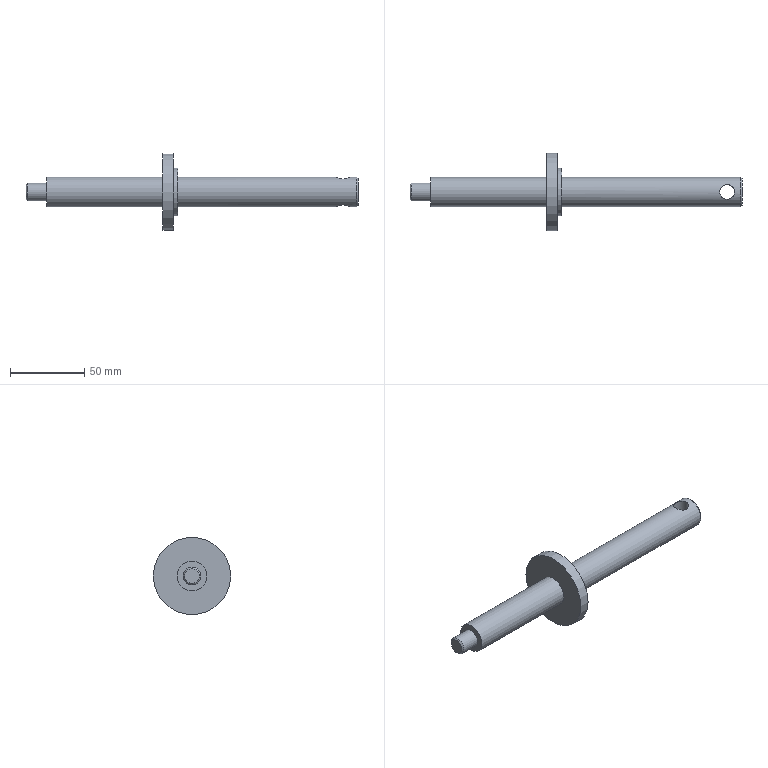Part | NX | features DATUM_CSYS 3, SKETCH 2, CHAMFER 1, EXTRUDE 1, HOLE PACKAGE 1, SIMPLE HOLE 1, SWP104 1, SYMBOLIC_THREAD 1 | 1 solid | 17 faces | box 223 x 52 x 52 mm | volume 79707 mm3 | cylinder 7 | plane 6 | cone 3 | spline 1 | commonest cylinder face diameters 20 x2 5 x1 10 x1 12 x1 32 x1 52 x1
STEP:
#1=CARTESIAN_POINT('',(222.,-10.,0.));
#2=VERTEX_POINT('',#1);
#3=CARTESIAN_POINT('',(222.,0.,0.));
#4=DIRECTION('',(-1.,0.,0.));
#5=DIRECTION('',(0.,-1.,0.));
#6=AXIS2_PLACEMENT_3D('',#3,#4,#5);
#7=CIRCLE('',#6,10.);
#8=EDGE_CURVE('',#2,#2,#7,.T.);
#9=ORIENTED_EDGE('',*,*,#8,.T.);
#10=EDGE_LOOP('',(#9));
#11=FACE_BOUND('',#10,.T.);
#12=CARTESIAN_POINT('',(102.,10.,0.));
#13=VERTEX_POINT('',#12);
#14=CARTESIAN_POINT('',(102.,0.,0.));
#15=DIRECTION('',(1.,0.,0.));
#16=DIRECTION('',(0.,1.,0.));
#17=AXIS2_PLACEMENT_3D('',#14,#15,#16);
#18=CIRCLE('',#17,10.);
#19=EDGE_CURVE('',#13,#13,#18,.T.);
#20=ORIENTED_EDGE('',*,*,#19,.T.);
#21=EDGE_LOOP('',(#20));
#22=FACE_BOUND('',#21,.T.);
#23=CARTESIAN_POINT('',(208.,0.,-10.));
#24=VERTEX_POINT('',#23);
#25=CARTESIAN_POINT('',(208.277,-2.001,-9.858));
#26=CARTESIAN_POINT('',(207.724,0.6768,-10.148));
#27=CARTESIAN_POINT('',(209.099,3.912,-9.377));
#28=CARTESIAN_POINT('',(212.31,5.272,-8.49));
#29=CARTESIAN_POINT('',(214.988,4.729,-8.824));
#30=CARTESIAN_POINT('',(217.159,3.276,-9.538));
#31=CARTESIAN_POINT('',(218.551,0.01854,-10.309));
#32=CARTESIAN_POINT('',(216.914,-3.918,-9.379));
#33=CARTESIAN_POINT('',(213.019,-5.545,-8.305));
#34=CARTESIAN_POINT('',(209.738,-4.174,-9.187));
#35=CARTESIAN_POINT('',(208.277,-2.001,-9.858));
#36=CARTESIAN_POINT('',(207.724,0.6768,-10.148));
#37=CARTESIAN_POINT('',(209.099,3.912,-9.377));
#38=B_SPLINE_CURVE_WITH_KNOTS('',3,(#25,#26,#27,#28,#29,#30,#31,#32,#33,#34,#35,#36,#37),.UNSPECIFIED.,.T.,.F.,(1,1,1,1,1,1,1,1,1,1,1,1,1,1,1,1,1),(-0.007946,-0.003973,-0.001986,0.,0.003973,0.007946,0.009932,0.01192,0.01589,0.01986,0.02384,0.02781,0.0298,0.03178,0.03575,0.03973,0.04171),.UNSPECIFIED.);
#39=EDGE_CURVE('',#24,#24,#38,.T.);
#40=ORIENTED_EDGE('',*,*,#39,.F.);
#41=EDGE_LOOP('',(#40));
#42=FACE_BOUND('',#41,.T.);
#43=CARTESIAN_POINT('',(208.,0.,10.));
#44=VERTEX_POINT('',#43);
#45=CARTESIAN_POINT('',(208.277,2.001,9.858));
#46=CARTESIAN_POINT('',(207.724,-0.6768,10.148));
#47=CARTESIAN_POINT('',(209.099,-3.912,9.377));
#48=CARTESIAN_POINT('',(212.31,-5.272,8.49));
#49=CARTESIAN_POINT('',(214.988,-4.729,8.824));
#50=CARTESIAN_POINT('',(217.159,-3.276,9.538));
#51=CARTESIAN_POINT('',(218.551,-0.01854,10.309));
#52=CARTESIAN_POINT('',(216.914,3.918,9.379));
#53=CARTESIAN_POINT('',(213.019,5.545,8.305));
#54=CARTESIAN_POINT('',(209.738,4.174,9.187));
#55=CARTESIAN_POINT('',(208.277,2.001,9.858));
#56=CARTESIAN_POINT('',(207.724,-0.6768,10.148));
#57=CARTESIAN_POINT('',(209.099,-3.912,9.377));
#58=B_SPLINE_CURVE_WITH_KNOTS('',3,(#45,#46,#47,#48,#49,#50,#51,#52,#53,#54,#55,#56,#57),.UNSPECIFIED.,.T.,.F.,(1,1,1,1,1,1,1,1,1,1,1,1,1,1,1,1,1),(-0.007946,-0.003973,-0.001986,0.,0.003973,0.007946,0.009932,0.01192,0.01589,0.01986,0.02384,0.02781,0.0298,0.03178,0.03575,0.03973,0.04171),.UNSPECIFIED.);
#59=EDGE_CURVE('',#44,#44,#58,.T.);
#60=ORIENTED_EDGE('',*,*,#59,.F.);
#61=EDGE_LOOP('',(#60));
#62=FACE_BOUND('',#61,.T.);
#63=CARTESIAN_POINT('',(0.,0.,0.));
#64=DIRECTION('',(1.,0.,0.));
#65=DIRECTION('',(0.,1.,0.));
#66=AXIS2_PLACEMENT_3D('',#63,#64,#65);
#67=CYLINDRICAL_SURFACE('',#66,10.);
#68=ADVANCED_FACE('',(#11,#22,#42,#62),#67,.T.);
#69=CARTESIAN_POINT('',(0.,5.,0.));
#70=VERTEX_POINT('',#69);
#71=CARTESIAN_POINT('',(0.,0.,0.));
#72=DIRECTION('',(1.,0.,0.));
#73=DIRECTION('',(0.,1.,0.));
#74=AXIS2_PLACEMENT_3D('',#71,#72,#73);
#75=CIRCLE('',#74,5.);
#76=EDGE_CURVE('',#70,#70,#75,.F.);
#77=ORIENTED_EDGE('',*,*,#76,.T.);
#78=EDGE_LOOP('',(#77));
#79=FACE_BOUND('',#78,.T.);
#80=CARTESIAN_POINT('',(0.,0.,0.));
#81=DIRECTION('',(1.,0.,0.));
#82=DIRECTION('',(0.,1.,0.));
#83=AXIS2_PLACEMENT_3D('',#80,#81,#82);
#84=PLANE('',#83);
#85=ADVANCED_FACE('',(#79),#84,.F.);
#86=CARTESIAN_POINT('',(1.,6.,0.));
#87=VERTEX_POINT('',#86);
#88=CARTESIAN_POINT('',(1.,0.,0.));
#89=DIRECTION('',(1.,0.,0.));
#90=DIRECTION('',(0.,1.,0.));
#91=AXIS2_PLACEMENT_3D('',#88,#89,#90);
#92=CIRCLE('',#91,6.);
#93=EDGE_CURVE('',#87,#87,#92,.T.);
#94=ORIENTED_EDGE('',*,*,#93,.T.);
#95=EDGE_LOOP('',(#94));
#96=FACE_BOUND('',#95,.T.);
#97=CARTESIAN_POINT('',(14.,6.,0.));
#98=VERTEX_POINT('',#97);
#99=CARTESIAN_POINT('',(14.,0.,0.));
#100=DIRECTION('',(1.,0.,0.));
#101=DIRECTION('',(0.,1.,0.));
#102=AXIS2_PLACEMENT_3D('',#99,#100,#101);
#103=CIRCLE('',#102,6.);
#104=EDGE_CURVE('',#98,#98,#103,.T.);
#105=ORIENTED_EDGE('',*,*,#104,.F.);
#106=EDGE_LOOP('',(#105));
#107=FACE_BOUND('',#106,.T.);
#108=CARTESIAN_POINT('',(0.,0.,0.));
#109=DIRECTION('',(1.,0.,0.));
#110=DIRECTION('',(0.,1.,0.));
#111=AXIS2_PLACEMENT_3D('',#108,#109,#110);
#112=CYLINDRICAL_SURFACE('',#111,6.);
#113=ADVANCED_FACE('',(#96,#107),#112,.T.);
#114=CARTESIAN_POINT('',(14.,10.,0.));
#115=VERTEX_POINT('',#114);
#116=CARTESIAN_POINT('',(14.,0.,0.));
#117=DIRECTION('',(1.,0.,0.));
#118=DIRECTION('',(0.,1.,0.));
#119=AXIS2_PLACEMENT_3D('',#116,#117,#118);
#120=CIRCLE('',#119,10.);
#121=EDGE_CURVE('',#115,#115,#120,.T.);
#122=ORIENTED_EDGE('',*,*,#121,.F.);
#123=EDGE_LOOP('',(#122));
#124=FACE_BOUND('',#123,.T.);
#125=ORIENTED_EDGE('',*,*,#104,.T.);
#126=EDGE_LOOP('',(#125));
#127=FACE_BOUND('',#126,.T.);
#128=CARTESIAN_POINT('',(14.,6.,0.));
#129=DIRECTION('',(1.,0.,0.));
#130=DIRECTION('',(0.,1.,0.));
#131=AXIS2_PLACEMENT_3D('',#128,#129,#130);
#132=PLANE('',#131);
#133=ADVANCED_FACE('',(#124,#127),#132,.F.);
#134=CARTESIAN_POINT('',(92.,10.,0.));
#135=VERTEX_POINT('',#134);
#136=CARTESIAN_POINT('',(92.,0.,0.));
#137=DIRECTION('',(1.,0.,0.));
#138=DIRECTION('',(0.,1.,0.));
#139=AXIS2_PLACEMENT_3D('',#136,#137,#138);
#140=CIRCLE('',#139,10.);
#141=EDGE_CURVE('',#135,#135,#140,.T.);
#142=ORIENTED_EDGE('',*,*,#141,.F.);
#143=EDGE_LOOP('',(#142));
#144=FACE_BOUND('',#143,.T.);
#145=ORIENTED_EDGE('',*,*,#121,.T.);
#146=EDGE_LOOP('',(#145));
#147=FACE_BOUND('',#146,.T.);
#148=CARTESIAN_POINT('',(0.,0.,0.));
#149=DIRECTION('',(1.,0.,0.));
#150=DIRECTION('',(0.,1.,0.));
#151=AXIS2_PLACEMENT_3D('',#148,#149,#150);
#152=CYLINDRICAL_SURFACE('',#151,10.);
#153=ADVANCED_FACE('',(#144,#147),#152,.T.);
#154=CARTESIAN_POINT('',(92.,26.,0.));
#155=VERTEX_POINT('',#154);
#156=CARTESIAN_POINT('',(92.,0.,0.));
#157=DIRECTION('',(1.,0.,0.));
#158=DIRECTION('',(0.,1.,0.));
#159=AXIS2_PLACEMENT_3D('',#156,#157,#158);
#160=CIRCLE('',#159,26.);
#161=EDGE_CURVE('',#155,#155,#160,.T.);
#162=ORIENTED_EDGE('',*,*,#161,.F.);
#163=EDGE_LOOP('',(#162));
#164=FACE_BOUND('',#163,.T.);
#165=ORIENTED_EDGE('',*,*,#141,.T.);
#166=EDGE_LOOP('',(#165));
#167=FACE_BOUND('',#166,.T.);
#168=CARTESIAN_POINT('',(92.,10.,0.));
#169=DIRECTION('',(1.,0.,0.));
#170=DIRECTION('',(0.,1.,0.));
#171=AXIS2_PLACEMENT_3D('',#168,#169,#170);
#172=PLANE('',#171);
#173=ADVANCED_FACE('',(#164,#167),#172,.F.);
#174=CARTESIAN_POINT('',(99.,26.,0.));
#175=VERTEX_POINT('',#174);
#176=CARTESIAN_POINT('',(99.,0.,0.));
#177=DIRECTION('',(1.,0.,0.));
#178=DIRECTION('',(0.,1.,0.));
#179=AXIS2_PLACEMENT_3D('',#176,#177,#178);
#180=CIRCLE('',#179,26.);
#181=EDGE_CURVE('',#175,#175,#180,.T.);
#182=ORIENTED_EDGE('',*,*,#181,.F.);
#183=EDGE_LOOP('',(#182));
#184=FACE_BOUND('',#183,.T.);
#185=ORIENTED_EDGE('',*,*,#161,.T.);
#186=EDGE_LOOP('',(#185));
#187=FACE_BOUND('',#186,.T.);
#188=CARTESIAN_POINT('',(0.,0.,0.));
#189=DIRECTION('',(1.,0.,0.));
#190=DIRECTION('',(0.,1.,0.));
#191=AXIS2_PLACEMENT_3D('',#188,#189,#190);
#192=CYLINDRICAL_SURFACE('',#191,26.);
#193=ADVANCED_FACE('',(#184,#187),#192,.T.);
#194=CARTESIAN_POINT('',(99.,16.,0.));
#195=VERTEX_POINT('',#194);
#196=CARTESIAN_POINT('',(99.,0.,0.));
#197=DIRECTION('',(1.,0.,0.));
#198=DIRECTION('',(0.,1.,0.));
#199=AXIS2_PLACEMENT_3D('',#196,#197,#198);
#200=CIRCLE('',#199,16.);
#201=EDGE_CURVE('',#195,#195,#200,.T.);
#202=ORIENTED_EDGE('',*,*,#201,.F.);
#203=EDGE_LOOP('',(#202));
#204=FACE_BOUND('',#203,.T.);
#205=ORIENTED_EDGE('',*,*,#181,.T.);
#206=EDGE_LOOP('',(#205));
#207=FACE_BOUND('',#206,.T.);
#208=CARTESIAN_POINT('',(99.,26.,0.));
#209=DIRECTION('',(-1.,0.,0.));
#210=DIRECTION('',(0.,-1.,0.));
#211=AXIS2_PLACEMENT_3D('',#208,#209,#210);
#212=PLANE('',#211);
#213=ADVANCED_FACE('',(#204,#207),#212,.F.);
#214=CARTESIAN_POINT('',(102.,16.,0.));
#215=VERTEX_POINT('',#214);
#216=CARTESIAN_POINT('',(102.,0.,0.));
#217=DIRECTION('',(1.,0.,0.));
#218=DIRECTION('',(0.,1.,0.));
#219=AXIS2_PLACEMENT_3D('',#216,#217,#218);
#220=CIRCLE('',#219,16.);
#221=EDGE_CURVE('',#215,#215,#220,.T.);
#222=ORIENTED_EDGE('',*,*,#221,.F.);
#223=EDGE_LOOP('',(#222));
#224=FACE_BOUND('',#223,.T.);
#225=ORIENTED_EDGE('',*,*,#201,.T.);
#226=EDGE_LOOP('',(#225));
#227=FACE_BOUND('',#226,.T.);
#228=CARTESIAN_POINT('',(0.,0.,0.));
#229=DIRECTION('',(1.,0.,0.));
#230=DIRECTION('',(0.,1.,0.));
#231=AXIS2_PLACEMENT_3D('',#228,#229,#230);
#232=CYLINDRICAL_SURFACE('',#231,16.);
#233=ADVANCED_FACE('',(#224,#227),#232,.T.);
#234=ORIENTED_EDGE('',*,*,#19,.F.);
#235=EDGE_LOOP('',(#234));
#236=FACE_BOUND('',#235,.T.);
#237=ORIENTED_EDGE('',*,*,#221,.T.);
#238=EDGE_LOOP('',(#237));
#239=FACE_BOUND('',#238,.T.);
#240=CARTESIAN_POINT('',(102.,16.,0.));
#241=DIRECTION('',(-1.,0.,0.));
#242=DIRECTION('',(0.,-1.,0.));
#243=AXIS2_PLACEMENT_3D('',#240,#241,#242);
#244=PLANE('',#243);
#245=ADVANCED_FACE('',(#236,#239),#244,.F.);
#246=CARTESIAN_POINT('',(223.,-3.,0.));
#247=VERTEX_POINT('',#246);
#248=CARTESIAN_POINT('',(223.,0.,0.));
#249=DIRECTION('',(-1.,0.,0.));
#250=DIRECTION('',(0.,-1.,0.));
#251=AXIS2_PLACEMENT_3D('',#248,#249,#250);
#252=CIRCLE('',#251,3.);
#253=EDGE_CURVE('',#247,#247,#252,.T.);
#254=ORIENTED_EDGE('',*,*,#253,.T.);
#255=EDGE_LOOP('',(#254));
#256=FACE_BOUND('',#255,.T.);
#257=CARTESIAN_POINT('',(223.,-9.,0.));
#258=VERTEX_POINT('',#257);
#259=CARTESIAN_POINT('',(223.,0.,0.));
#260=DIRECTION('',(-1.,0.,0.));
#261=DIRECTION('',(0.,-1.,0.));
#262=AXIS2_PLACEMENT_3D('',#259,#260,#261);
#263=CIRCLE('',#262,9.);
#264=EDGE_CURVE('',#258,#258,#263,.F.);
#265=ORIENTED_EDGE('',*,*,#264,.T.);
#266=EDGE_LOOP('',(#265));
#267=FACE_BOUND('',#266,.T.);
#268=CARTESIAN_POINT('',(223.,10.,0.));
#269=DIRECTION('',(-1.,0.,0.));
#270=DIRECTION('',(0.,-1.,0.));
#271=AXIS2_PLACEMENT_3D('',#268,#269,#270);
#272=PLANE('',#271);
#273=ADVANCED_FACE('',(#256,#267),#272,.F.);
#274=ORIENTED_EDGE('',*,*,#8,.F.);
#275=EDGE_LOOP('',(#274));
#276=FACE_BOUND('',#275,.T.);
#277=ORIENTED_EDGE('',*,*,#264,.F.);
#278=EDGE_LOOP('',(#277));
#279=FACE_BOUND('',#278,.T.);
#280=CARTESIAN_POINT('',(223.,0.,0.));
#281=DIRECTION('',(-1.,0.,0.));
#282=DIRECTION('',(0.,-1.,0.));
#283=AXIS2_PLACEMENT_3D('',#280,#281,#282);
#284=CONICAL_SURFACE('',#283,9.,0.7854);
#285=ADVANCED_FACE('',(#276,#279),#284,.T.);
#286=ORIENTED_EDGE('',*,*,#76,.F.);
#287=EDGE_LOOP('',(#286));
#288=FACE_BOUND('',#287,.T.);
#289=ORIENTED_EDGE('',*,*,#93,.F.);
#290=EDGE_LOOP('',(#289));
#291=FACE_BOUND('',#290,.T.);
#292=CARTESIAN_POINT('',(1.,0.,0.));
#293=DIRECTION('',(1.,0.,0.));
#294=DIRECTION('',(0.,1.,0.));
#295=AXIS2_PLACEMENT_3D('',#292,#293,#294);
#296=CONICAL_SURFACE('',#295,6.,0.7854);
#297=ADVANCED_FACE('',(#288,#291),#296,.T.);
#298=CARTESIAN_POINT('',(217.187,-2.733,0.));
#299=VERTEX_POINT('',#298);
#300=CARTESIAN_POINT('',(217.301,-2.566,1.32));
#301=CARTESIAN_POINT('',(217.134,-2.81,0.043));
#302=CARTESIAN_POINT('',(217.283,-2.593,-1.23));
#303=CARTESIAN_POINT('',(217.596,-2.024,-2.271));
#304=CARTESIAN_POINT('',(217.903,-1.148,-2.992));
#305=CARTESIAN_POINT('',(218.041,-0.06264,-3.292));
#306=CARTESIAN_POINT('',(217.93,1.032,-3.052));
#307=CARTESIAN_POINT('',(217.633,1.942,-2.368));
#308=CARTESIAN_POINT('',(217.308,2.554,-1.343));
#309=CARTESIAN_POINT('',(217.135,2.809,-0.07027));
#310=CARTESIAN_POINT('',(217.276,2.604,1.207));
#311=CARTESIAN_POINT('',(217.595,2.025,2.27));
#312=CARTESIAN_POINT('',(217.903,1.148,2.992));
#313=CARTESIAN_POINT('',(218.042,0.06158,3.292));
#314=CARTESIAN_POINT('',(217.929,-1.034,3.051));
#315=CARTESIAN_POINT('',(217.632,-1.944,2.366));
#316=CARTESIAN_POINT('',(217.301,-2.566,1.32));
#317=CARTESIAN_POINT('',(217.134,-2.81,0.043));
#318=CARTESIAN_POINT('',(217.283,-2.593,-1.23));
#319=B_SPLINE_CURVE_WITH_KNOTS('',3,(#300,#301,#302,#303,#304,#305,#306,#307,#308,#309,#310,#311,#312,#313,#314,#315,#316,#317,#318),.UNSPECIFIED.,.T.,.F.,(1,1,1,1,1,1,1,1,1,1,1,1,1,1,1,1,1,1,1,1,1,1,1),(-0.1908,-0.1283,-0.06579,0.,0.05937,0.1217,0.1842,0.2467,0.3092,0.3717,0.4342,0.4967,0.5592,0.6217,0.6842,0.7467,0.8092,0.8717,0.9342,1.,1.059,1.122,1.184),.UNSPECIFIED.);
#320=EDGE_CURVE('',#299,#299,#319,.T.);
#321=ORIENTED_EDGE('',*,*,#320,.T.);
#322=EDGE_LOOP('',(#321));
#323=FACE_BOUND('',#322,.T.);
#324=ORIENTED_EDGE('',*,*,#39,.T.);
#325=EDGE_LOOP('',(#324));
#326=FACE_BOUND('',#325,.T.);
#327=ORIENTED_EDGE('',*,*,#59,.T.);
#328=EDGE_LOOP('',(#327));
#329=FACE_BOUND('',#328,.T.);
#330=CARTESIAN_POINT('',(213.,0.,64.));
#331=DIRECTION('',(0.,0.,-1.));
#332=DIRECTION('',(-1.,0.,0.));
#333=AXIS2_PLACEMENT_3D('',#330,#331,#332);
#334=CYLINDRICAL_SURFACE('',#333,5.);
#335=ADVANCED_FACE('',(#323,#326,#329),#334,.F.);
#336=CARTESIAN_POINT('',(217.906,-2.5,0.));
#337=VERTEX_POINT('',#336);
#338=CARTESIAN_POINT('',(217.931,-2.476,-0.4847));
#339=CARTESIAN_POINT('',(217.895,-2.51,-0.01351));
#340=CARTESIAN_POINT('',(217.925,-2.482,0.4271));
#341=CARTESIAN_POINT('',(218.053,-2.32,0.9666));
#342=CARTESIAN_POINT('',(218.158,-2.177,1.253));
#343=CARTESIAN_POINT('',(218.451,-1.723,1.893));
#344=CARTESIAN_POINT('',(218.77,-0.9129,2.395));
#345=CARTESIAN_POINT('',(218.893,-0.06401,2.539));
#346=CARTESIAN_POINT('',(218.804,0.7449,2.442));
#347=CARTESIAN_POINT('',(218.538,1.561,2.039));
#348=CARTESIAN_POINT('',(218.198,2.121,1.357));
#349=CARTESIAN_POINT('',(218.078,2.286,1.043));
#350=CARTESIAN_POINT('',(217.937,2.468,0.5114));
#351=CARTESIAN_POINT('',(217.895,2.51,0.04032));
#352=CARTESIAN_POINT('',(217.92,2.488,-0.4006));
#353=CARTESIAN_POINT('',(218.051,2.322,-0.962));
#354=CARTESIAN_POINT('',(218.158,2.177,-1.254));
#355=CARTESIAN_POINT('',(218.452,1.721,-1.895));
#356=CARTESIAN_POINT('',(218.77,0.9117,-2.395));
#357=CARTESIAN_POINT('',(218.893,0.06296,-2.539));
#358=CARTESIAN_POINT('',(218.804,-0.7453,-2.441));
#359=CARTESIAN_POINT('',(218.538,-1.561,-2.039));
#360=CARTESIAN_POINT('',(218.199,-2.12,-1.358));
#361=CARTESIAN_POINT('',(218.076,-2.288,-1.039));
#362=CARTESIAN_POINT('',(217.931,-2.476,-0.4847));
#363=CARTESIAN_POINT('',(217.895,-2.51,-0.01351));
#364=CARTESIAN_POINT('',(217.925,-2.482,0.4271));
#365=B_SPLINE_CURVE_WITH_KNOTS('',3,(#338,#339,#340,#341,#342,#343,#344,#345,#346,#347,#348,#349,#350,#351,#352,#353,#354,#355,#356,#357,#358,#359,#360,#361,#362,#363,#364),.UNSPECIFIED.,.T.,.F.,(1,1,1,1,1,1,1,1,1,1,1,1,1,1,1,1,1,1,1,1,1,1,1,1,1,1,1,1,1,1,1),(-0.09876,-0.06595,-0.03298,0.,0.02969,0.05937,0.09055,0.1217,0.1827,0.2436,0.306,0.3684,0.4012,0.434,0.4654,0.4967,0.528,0.5592,0.5905,0.6217,0.6826,0.7436,0.806,0.8684,0.9012,0.934,0.967,1.,1.03,1.059,1.091),.UNSPECIFIED.);
#366=EDGE_CURVE('',#337,#337,#365,.T.);
#367=ORIENTED_EDGE('',*,*,#366,.T.);
#368=EDGE_LOOP('',(#367));
#369=FACE_BOUND('',#368,.T.);
#370=CARTESIAN_POINT('',(222.5,-2.5,0.));
#371=VERTEX_POINT('',#370);
#372=CARTESIAN_POINT('',(222.5,0.,0.));
#373=DIRECTION('',(-1.,0.,0.));
#374=DIRECTION('',(0.,-1.,0.));
#375=AXIS2_PLACEMENT_3D('',#372,#373,#374);
#376=CIRCLE('',#375,2.5);
#377=EDGE_CURVE('',#371,#371,#376,.F.);
#378=ORIENTED_EDGE('',*,*,#377,.T.);
#379=EDGE_LOOP('',(#378));
#380=FACE_BOUND('',#379,.T.);
#381=CARTESIAN_POINT('',(223.,0.,0.));
#382=DIRECTION('',(-1.,0.,0.));
#383=DIRECTION('',(0.,-1.,0.));
#384=AXIS2_PLACEMENT_3D('',#381,#382,#383);
#385=CYLINDRICAL_SURFACE('',#384,2.5);
#386=ADVANCED_FACE('',(#369,#380),#385,.F.);
#387=ORIENTED_EDGE('',*,*,#377,.F.);
#388=EDGE_LOOP('',(#387));
#389=FACE_BOUND('',#388,.T.);
#390=ORIENTED_EDGE('',*,*,#253,.F.);
#391=EDGE_LOOP('',(#390));
#392=FACE_BOUND('',#391,.T.);
#393=CARTESIAN_POINT('',(223.,0.,0.));
#394=DIRECTION('',(1.,0.,0.));
#395=DIRECTION('',(0.,1.,0.));
#396=AXIS2_PLACEMENT_3D('',#393,#394,#395);
#397=CONICAL_SURFACE('',#396,3.,0.7854);
#398=ADVANCED_FACE('',(#389,#392),#397,.F.);
#399=ORIENTED_EDGE('',*,*,#320,.F.);
#400=EDGE_LOOP('',(#399));
#401=FACE_BOUND('',#400,.T.);
#402=ORIENTED_EDGE('',*,*,#366,.F.);
#403=EDGE_LOOP('',(#402));
#404=FACE_BOUND('',#403,.T.);
#405=CARTESIAN_POINT('',(217.905,-2.501,-0.674));
#406=CARTESIAN_POINT('',(217.906,-2.499,0.674));
#407=CARTESIAN_POINT('',(218.156,-2.22,1.313));
#408=CARTESIAN_POINT('',(218.649,-1.319,2.219));
#409=CARTESIAN_POINT('',(218.86,-0.6705,2.501));
#410=CARTESIAN_POINT('',(218.858,0.6761,2.499));
#411=CARTESIAN_POINT('',(218.648,1.32,2.217));
#412=CARTESIAN_POINT('',(218.156,2.222,1.313));
#413=CARTESIAN_POINT('',(217.905,2.501,0.6725));
#414=CARTESIAN_POINT('',(217.907,2.499,-0.6778));
#415=CARTESIAN_POINT('',(218.158,2.218,-1.316));
#416=CARTESIAN_POINT('',(218.649,1.317,-2.22));
#417=CARTESIAN_POINT('',(218.86,0.6689,-2.502));
#418=CARTESIAN_POINT('',(218.857,-0.6764,-2.498));
#419=CARTESIAN_POINT('',(218.648,-1.319,-2.217));
#420=CARTESIAN_POINT('',(218.156,-2.221,-1.314));
#421=CARTESIAN_POINT('',(217.905,-2.501,-0.674));
#422=CARTESIAN_POINT('',(217.906,-2.499,0.674));
#423=CARTESIAN_POINT('',(217.186,-2.734,-0.8633));
#424=CARTESIAN_POINT('',(217.187,-2.732,0.8633));
#425=CARTESIAN_POINT('',(217.401,-2.427,1.682));
#426=CARTESIAN_POINT('',(217.821,-1.442,2.843));
#427=CARTESIAN_POINT('',(218.001,-0.7331,3.204));
#428=CARTESIAN_POINT('',(217.999,0.7392,3.201));
#429=CARTESIAN_POINT('',(217.82,1.443,2.84));
#430=CARTESIAN_POINT('',(217.4,2.429,1.682));
#431=CARTESIAN_POINT('',(217.186,2.735,0.8615));
#432=CARTESIAN_POINT('',(217.188,2.732,-0.8683));
#433=CARTESIAN_POINT('',(217.402,2.425,-1.686));
#434=CARTESIAN_POINT('',(217.821,1.44,-2.844));
#435=CARTESIAN_POINT('',(218.001,0.7313,-3.205));
#436=CARTESIAN_POINT('',(217.999,-0.7395,-3.2));
#437=CARTESIAN_POINT('',(217.82,-1.442,-2.84));
#438=CARTESIAN_POINT('',(217.401,-2.428,-1.683));
#439=CARTESIAN_POINT('',(217.186,-2.734,-0.8633));
#440=CARTESIAN_POINT('',(217.187,-2.732,0.8633));
#441=B_SPLINE_SURFACE_WITH_KNOTS('',1,3,((#405,#406,#407,#408,#409,#410,#411,#412,#413,#414,#415,#416,#417,#418,#419,#420,#421,#422),(#423,#424,#425,#426,#427,#428,#429,#430,#431,#432,#433,#434,#435,#436,#437,#438,#439,#440)),.RULED_SURF.,.F.,.T.,.F.,(2,2),(2,2,2,2,2,2,2,2,2,2,2),(0.,1.),(-0.02178,-0.01922,-0.01666,-0.01411,-0.01155,-0.008991,-0.006434,-0.003876,-0.001319,0.001238,0.003796),.UNSPECIFIED.);
#442=ADVANCED_FACE('',(#401,#404),#441,.T.);
#443=CLOSED_SHELL('',(#68,#85,#113,#133,#153,#173,#193,#213,#233,#245,#273,#285,#297,#335,#386,#398,#442));
#444=MANIFOLD_SOLID_BREP('',#443);
#445=(LENGTH_UNIT()NAMED_UNIT(*)SI_UNIT(.MILLI.,.METRE.));
#446=UNCERTAINTY_MEASURE_WITH_UNIT(LENGTH_MEASURE(0.0508),#445,'','');
#447=(NAMED_UNIT(*)PLANE_ANGLE_UNIT()SI_UNIT($,.RADIAN.));
#448=(NAMED_UNIT(*)SI_UNIT($,.STERADIAN.)SOLID_ANGLE_UNIT());
#449=(GEOMETRIC_REPRESENTATION_CONTEXT(3)GLOBAL_UNCERTAINTY_ASSIGNED_CONTEXT((#446))GLOBAL_UNIT_ASSIGNED_CONTEXT((#445,#447,#448))REPRESENTATION_CONTEXT('',''));
#450=ADVANCED_BREP_SHAPE_REPRESENTATION('',(#444),#449);